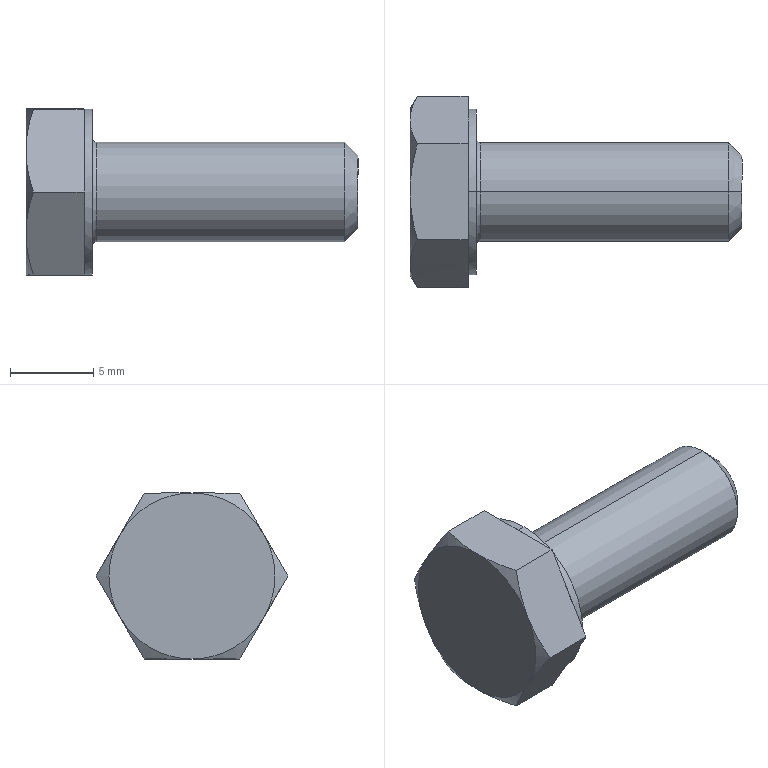Part | SolidWorks | features BaseBody 1 | 1 solid | 29 faces | box 20 x 11.547 x 10 mm | volume 788.422 mm3 | plane 15 | cone 8 | cylinder 4 | torus 2 | commonest cylinder face diameters 6 x2 10 x2
STEP:
#1=CARTESIAN_POINT('',(4.25,0.,3.));
#2=VERTEX_POINT('',#1);
#3=CARTESIAN_POINT('',(4.,0.,3.25));
#4=VERTEX_POINT('',#3);
#5=CARTESIAN_POINT('',(4.25,0.,3.25));
#6=DIRECTION('',(0.,1.,0.));
#7=DIRECTION('',(-1.,0.,0.));
#8=AXIS2_PLACEMENT_3D('',#5,#6,#7);
#9=CIRCLE('',#8,0.25);
#10=EDGE_CURVE('',#2,#4,#9,.T.);
#11=ORIENTED_EDGE('',*,*,#10,.F.);
#12=CARTESIAN_POINT('',(4.25,0.,-3.));
#13=VERTEX_POINT('',#12);
#14=CARTESIAN_POINT('',(4.25,0.,0.));
#15=DIRECTION('',(1.,0.,0.));
#16=DIRECTION('',(0.,0.,-1.));
#17=AXIS2_PLACEMENT_3D('',#14,#15,#16);
#18=CIRCLE('',#17,3.);
#19=EDGE_CURVE('',#13,#2,#18,.T.);
#20=ORIENTED_EDGE('',*,*,#19,.F.);
#21=CARTESIAN_POINT('',(4.,0.,-3.25));
#22=VERTEX_POINT('',#21);
#23=CARTESIAN_POINT('',(4.25,0.,-3.25));
#24=DIRECTION('',(0.,-1.,0.));
#25=DIRECTION('',(1.,0.,0.));
#26=AXIS2_PLACEMENT_3D('',#23,#24,#25);
#27=CIRCLE('',#26,0.25);
#28=EDGE_CURVE('',#13,#22,#27,.T.);
#29=ORIENTED_EDGE('',*,*,#28,.T.);
#30=CARTESIAN_POINT('',(4.,0.,0.));
#31=DIRECTION('',(-1.,0.,0.));
#32=DIRECTION('',(0.,0.,-1.));
#33=AXIS2_PLACEMENT_3D('',#30,#31,#32);
#34=CIRCLE('',#33,3.25);
#35=EDGE_CURVE('',#4,#22,#34,.T.);
#36=ORIENTED_EDGE('',*,*,#35,.F.);
#37=EDGE_LOOP('',(#11,#20,#29,#36));
#38=FACE_OUTER_BOUND('',#37,.T.);
#39=CARTESIAN_POINT('',(4.25,0.,0.));
#40=DIRECTION('',(1.,0.,0.));
#41=DIRECTION('',(0.,0.,-1.));
#42=AXIS2_PLACEMENT_3D('',#39,#40,#41);
#43=TOROIDAL_SURFACE('',#42,3.25,0.25);
#44=ADVANCED_FACE('',(#38),#43,.F.);
#45=CARTESIAN_POINT('',(20.,0.,-2.2));
#46=VERTEX_POINT('',#45);
#47=CARTESIAN_POINT('',(19.2,0.,-3.));
#48=VERTEX_POINT('',#47);
#49=CARTESIAN_POINT('',(19.2,0.,-3.));
#50=DIRECTION('',(-0.7071,0.,-0.7071));
#51=VECTOR('',#50,1000.);
#52=LINE('',#49,#51);
#53=EDGE_CURVE('',#46,#48,#52,.T.);
#54=ORIENTED_EDGE('',*,*,#53,.F.);
#55=CARTESIAN_POINT('',(20.,0.,2.2));
#56=VERTEX_POINT('',#55);
#57=CARTESIAN_POINT('',(20.,0.,0.));
#58=DIRECTION('',(1.,0.,0.));
#59=DIRECTION('',(0.,0.,1.));
#60=AXIS2_PLACEMENT_3D('',#57,#58,#59);
#61=CIRCLE('',#60,2.2);
#62=EDGE_CURVE('',#56,#46,#61,.T.);
#63=ORIENTED_EDGE('',*,*,#62,.F.);
#64=CARTESIAN_POINT('',(19.2,0.,3.));
#65=VERTEX_POINT('',#64);
#66=CARTESIAN_POINT('',(19.2,0.,3.));
#67=DIRECTION('',(-0.7071,0.,0.7071));
#68=VECTOR('',#67,1000.);
#69=LINE('',#66,#68);
#70=EDGE_CURVE('',#56,#65,#69,.T.);
#71=ORIENTED_EDGE('',*,*,#70,.T.);
#72=CARTESIAN_POINT('',(19.2,0.,0.));
#73=DIRECTION('',(-1.,0.,0.));
#74=DIRECTION('',(0.,0.,1.));
#75=AXIS2_PLACEMENT_3D('',#72,#73,#74);
#76=CIRCLE('',#75,3.);
#77=EDGE_CURVE('',#48,#65,#76,.T.);
#78=ORIENTED_EDGE('',*,*,#77,.F.);
#79=EDGE_LOOP('',(#54,#63,#71,#78));
#80=FACE_OUTER_BOUND('',#79,.T.);
#81=CARTESIAN_POINT('',(19.2,0.,0.));
#82=DIRECTION('',(-1.,0.,0.));
#83=DIRECTION('',(0.,0.,1.));
#84=AXIS2_PLACEMENT_3D('',#81,#82,#83);
#85=CONICAL_SURFACE('',#84,3.,0.7854);
#86=ADVANCED_FACE('',(#80),#85,.T.);
#87=CARTESIAN_POINT('',(4.,0.,0.));
#88=DIRECTION('',(-1.,0.,0.));
#89=DIRECTION('',(0.,0.,-1.));
#90=AXIS2_PLACEMENT_3D('',#87,#88,#89);
#91=CIRCLE('',#90,3.25);
#92=EDGE_CURVE('',#22,#4,#91,.T.);
#93=ORIENTED_EDGE('',*,*,#92,.T.);
#94=ORIENTED_EDGE('',*,*,#35,.T.);
#95=EDGE_LOOP('',(#93,#94));
#96=FACE_BOUND('',#95,.T.);
#97=CARTESIAN_POINT('',(4.,0.,5.));
#98=VERTEX_POINT('',#97);
#99=CARTESIAN_POINT('',(4.,0.,-5.));
#100=VERTEX_POINT('',#99);
#101=CARTESIAN_POINT('',(4.,0.,0.));
#102=DIRECTION('',(1.,0.,0.));
#103=DIRECTION('',(0.,0.,-1.));
#104=AXIS2_PLACEMENT_3D('',#101,#102,#103);
#105=CIRCLE('',#104,5.);
#106=EDGE_CURVE('',#98,#100,#105,.T.);
#107=ORIENTED_EDGE('',*,*,#106,.T.);
#108=CARTESIAN_POINT('',(4.,0.,0.));
#109=DIRECTION('',(1.,0.,0.));
#110=DIRECTION('',(0.,0.,-1.));
#111=AXIS2_PLACEMENT_3D('',#108,#109,#110);
#112=CIRCLE('',#111,5.);
#113=EDGE_CURVE('',#100,#98,#112,.T.);
#114=ORIENTED_EDGE('',*,*,#113,.T.);
#115=EDGE_LOOP('',(#107,#114));
#116=FACE_OUTER_BOUND('',#115,.T.);
#117=CARTESIAN_POINT('',(4.,0.,-10.));
#118=DIRECTION('',(1.,0.,0.));
#119=DIRECTION('',(0.,0.,-1.));
#120=AXIS2_PLACEMENT_3D('',#117,#118,#119);
#121=PLANE('',#120);
#122=ADVANCED_FACE('',(#96,#116),#121,.T.);
#123=CARTESIAN_POINT('',(0.,0.,-3.));
#124=DIRECTION('',(-1.,0.,0.));
#125=VECTOR('',#124,1000.);
#126=LINE('',#123,#125);
#127=EDGE_CURVE('',#48,#13,#126,.T.);
#128=ORIENTED_EDGE('',*,*,#127,.F.);
#129=ORIENTED_EDGE('',*,*,#77,.T.);
#130=CARTESIAN_POINT('',(0.,0.,3.));
#131=DIRECTION('',(-1.,0.,0.));
#132=VECTOR('',#131,1000.);
#133=LINE('',#130,#132);
#134=EDGE_CURVE('',#65,#2,#133,.T.);
#135=ORIENTED_EDGE('',*,*,#134,.T.);
#136=CARTESIAN_POINT('',(4.25,0.,0.));
#137=DIRECTION('',(1.,0.,0.));
#138=DIRECTION('',(0.,0.,-1.));
#139=AXIS2_PLACEMENT_3D('',#136,#137,#138);
#140=CIRCLE('',#139,3.);
#141=EDGE_CURVE('',#2,#13,#140,.T.);
#142=ORIENTED_EDGE('',*,*,#141,.T.);
#143=EDGE_LOOP('',(#128,#129,#135,#142));
#144=FACE_OUTER_BOUND('',#143,.T.);
#145=CARTESIAN_POINT('',(0.,0.,0.));
#146=DIRECTION('',(-1.,0.,0.));
#147=DIRECTION('',(0.,0.,1.));
#148=AXIS2_PLACEMENT_3D('',#145,#146,#147);
#149=CYLINDRICAL_SURFACE('',#148,3.);
#150=ADVANCED_FACE('',(#144),#149,.T.);
#151=ORIENTED_EDGE('',*,*,#62,.T.);
#152=CARTESIAN_POINT('',(20.,0.,0.));
#153=DIRECTION('',(1.,0.,0.));
#154=DIRECTION('',(0.,0.,1.));
#155=AXIS2_PLACEMENT_3D('',#152,#153,#154);
#156=CIRCLE('',#155,2.2);
#157=EDGE_CURVE('',#46,#56,#156,.T.);
#158=ORIENTED_EDGE('',*,*,#157,.T.);
#159=EDGE_LOOP('',(#151,#158));
#160=FACE_OUTER_BOUND('',#159,.T.);
#161=CARTESIAN_POINT('',(20.,0.,0.));
#162=DIRECTION('',(-1.,0.,0.));
#163=DIRECTION('',(0.,1.,0.));
#164=AXIS2_PLACEMENT_3D('',#161,#162,#163);
#165=PLANE('',#164);
#166=ADVANCED_FACE('',(#160),#165,.F.);
#167=CARTESIAN_POINT('',(3.5,0.,-5.));
#168=VERTEX_POINT('',#167);
#169=CARTESIAN_POINT('',(0.,0.,-5.));
#170=DIRECTION('',(-1.,0.,0.));
#171=VECTOR('',#170,1000.);
#172=LINE('',#169,#171);
#173=EDGE_CURVE('',#100,#168,#172,.T.);
#174=ORIENTED_EDGE('',*,*,#173,.F.);
#175=ORIENTED_EDGE('',*,*,#106,.F.);
#176=CARTESIAN_POINT('',(3.5,0.,5.));
#177=VERTEX_POINT('',#176);
#178=CARTESIAN_POINT('',(0.,0.,5.));
#179=DIRECTION('',(-1.,0.,0.));
#180=VECTOR('',#179,1000.);
#181=LINE('',#178,#180);
#182=EDGE_CURVE('',#98,#177,#181,.T.);
#183=ORIENTED_EDGE('',*,*,#182,.T.);
#184=CARTESIAN_POINT('',(3.5,-4.33,2.5));
#185=VERTEX_POINT('',#184);
#186=CARTESIAN_POINT('',(3.5,0.,0.));
#187=DIRECTION('',(-1.,0.,0.));
#188=DIRECTION('',(0.,0.,1.));
#189=AXIS2_PLACEMENT_3D('',#186,#187,#188);
#190=CIRCLE('',#189,5.);
#191=EDGE_CURVE('',#185,#177,#190,.T.);
#192=ORIENTED_EDGE('',*,*,#191,.F.);
#193=CARTESIAN_POINT('',(3.5,-4.33,-2.5));
#194=VERTEX_POINT('',#193);
#195=CARTESIAN_POINT('',(3.5,0.,0.));
#196=DIRECTION('',(-1.,0.,0.));
#197=DIRECTION('',(0.,0.,1.));
#198=AXIS2_PLACEMENT_3D('',#195,#196,#197);
#199=CIRCLE('',#198,5.);
#200=EDGE_CURVE('',#194,#185,#199,.T.);
#201=ORIENTED_EDGE('',*,*,#200,.F.);
#202=CARTESIAN_POINT('',(3.5,0.,0.));
#203=DIRECTION('',(-1.,0.,0.));
#204=DIRECTION('',(0.,0.,1.));
#205=AXIS2_PLACEMENT_3D('',#202,#203,#204);
#206=CIRCLE('',#205,5.);
#207=EDGE_CURVE('',#168,#194,#206,.T.);
#208=ORIENTED_EDGE('',*,*,#207,.F.);
#209=EDGE_LOOP('',(#174,#175,#183,#192,#201,#208));
#210=FACE_OUTER_BOUND('',#209,.T.);
#211=CARTESIAN_POINT('',(0.,0.,0.));
#212=DIRECTION('',(-1.,0.,0.));
#213=DIRECTION('',(0.,0.,1.));
#214=AXIS2_PLACEMENT_3D('',#211,#212,#213);
#215=CYLINDRICAL_SURFACE('',#214,5.);
#216=ADVANCED_FACE('',(#210),#215,.T.);
#217=CARTESIAN_POINT('',(3.5,-2.887,-5.));
#218=VERTEX_POINT('',#217);
#219=CARTESIAN_POINT('',(3.5,-2.887,-5.));
#220=DIRECTION('',(0.,0.5,-0.866));
#221=VECTOR('',#220,1000.);
#222=LINE('',#219,#221);
#223=EDGE_CURVE('',#194,#218,#222,.T.);
#224=ORIENTED_EDGE('',*,*,#223,.T.);
#225=CARTESIAN_POINT('',(3.5,2.887,-5.));
#226=DIRECTION('',(0.,1.,0.));
#227=VECTOR('',#226,1000.);
#228=LINE('',#225,#227);
#229=EDGE_CURVE('',#218,#168,#228,.T.);
#230=ORIENTED_EDGE('',*,*,#229,.T.);
#231=ORIENTED_EDGE('',*,*,#207,.T.);
#232=EDGE_LOOP('',(#224,#230,#231));
#233=FACE_OUTER_BOUND('',#232,.T.);
#234=CARTESIAN_POINT('',(3.5,5.,0.));
#235=DIRECTION('',(1.,0.,0.));
#236=DIRECTION('',(0.,0.,-1.));
#237=AXIS2_PLACEMENT_3D('',#234,#235,#236);
#238=PLANE('',#237);
#239=ADVANCED_FACE('',(#233),#238,.T.);
#240=CARTESIAN_POINT('',(3.5,-5.774,0.));
#241=VERTEX_POINT('',#240);
#242=CARTESIAN_POINT('',(3.5,-5.774,0.));
#243=DIRECTION('',(0.,-0.5,-0.866));
#244=VECTOR('',#243,1000.);
#245=LINE('',#242,#244);
#246=EDGE_CURVE('',#185,#241,#245,.T.);
#247=ORIENTED_EDGE('',*,*,#246,.T.);
#248=CARTESIAN_POINT('',(3.5,-2.887,-5.));
#249=DIRECTION('',(0.,0.5,-0.866));
#250=VECTOR('',#249,1000.);
#251=LINE('',#248,#250);
#252=EDGE_CURVE('',#241,#194,#251,.T.);
#253=ORIENTED_EDGE('',*,*,#252,.T.);
#254=ORIENTED_EDGE('',*,*,#200,.T.);
#255=EDGE_LOOP('',(#247,#253,#254));
#256=FACE_OUTER_BOUND('',#255,.T.);
#257=CARTESIAN_POINT('',(3.5,5.,0.));
#258=DIRECTION('',(1.,0.,0.));
#259=DIRECTION('',(0.,0.,-1.));
#260=AXIS2_PLACEMENT_3D('',#257,#258,#259);
#261=PLANE('',#260);
#262=ADVANCED_FACE('',(#256),#261,.T.);
#263=CARTESIAN_POINT('',(3.5,-2.887,5.));
#264=VERTEX_POINT('',#263);
#265=CARTESIAN_POINT('',(3.5,2.887,5.));
#266=DIRECTION('',(0.,-1.,0.));
#267=VECTOR('',#266,1000.);
#268=LINE('',#265,#267);
#269=EDGE_CURVE('',#177,#264,#268,.T.);
#270=ORIENTED_EDGE('',*,*,#269,.T.);
#271=CARTESIAN_POINT('',(3.5,-5.774,0.));
#272=DIRECTION('',(0.,-0.5,-0.866));
#273=VECTOR('',#272,1000.);
#274=LINE('',#271,#273);
#275=EDGE_CURVE('',#264,#185,#274,.T.);
#276=ORIENTED_EDGE('',*,*,#275,.T.);
#277=ORIENTED_EDGE('',*,*,#191,.T.);
#278=EDGE_LOOP('',(#270,#276,#277));
#279=FACE_OUTER_BOUND('',#278,.T.);
#280=CARTESIAN_POINT('',(3.5,5.,0.));
#281=DIRECTION('',(1.,0.,0.));
#282=DIRECTION('',(0.,0.,-1.));
#283=AXIS2_PLACEMENT_3D('',#280,#281,#282);
#284=PLANE('',#283);
#285=ADVANCED_FACE('',(#279),#284,.T.);
#286=CARTESIAN_POINT('',(3.5,4.33,2.5));
#287=VERTEX_POINT('',#286);
#288=CARTESIAN_POINT('',(3.5,2.887,5.));
#289=VERTEX_POINT('',#288);
#290=CARTESIAN_POINT('',(3.5,5.774,0.));
#291=DIRECTION('',(0.,-0.5,0.866));
#292=VECTOR('',#291,1000.);
#293=LINE('',#290,#292);
#294=EDGE_CURVE('',#287,#289,#293,.T.);
#295=ORIENTED_EDGE('',*,*,#294,.T.);
#296=CARTESIAN_POINT('',(3.5,2.887,5.));
#297=DIRECTION('',(0.,-1.,0.));
#298=VECTOR('',#297,1000.);
#299=LINE('',#296,#298);
#300=EDGE_CURVE('',#289,#177,#299,.T.);
#301=ORIENTED_EDGE('',*,*,#300,.T.);
#302=CARTESIAN_POINT('',(3.5,0.,0.));
#303=DIRECTION('',(-1.,0.,0.));
#304=DIRECTION('',(0.,0.,1.));
#305=AXIS2_PLACEMENT_3D('',#302,#303,#304);
#306=CIRCLE('',#305,5.);
#307=EDGE_CURVE('',#177,#287,#306,.T.);
#308=ORIENTED_EDGE('',*,*,#307,.T.);
#309=EDGE_LOOP('',(#295,#301,#308));
#310=FACE_OUTER_BOUND('',#309,.T.);
#311=CARTESIAN_POINT('',(3.5,5.,0.));
#312=DIRECTION('',(1.,0.,0.));
#313=DIRECTION('',(0.,0.,-1.));
#314=AXIS2_PLACEMENT_3D('',#311,#312,#313);
#315=PLANE('',#314);
#316=ADVANCED_FACE('',(#310),#315,.T.);
#317=CARTESIAN_POINT('',(3.5,4.33,-2.5));
#318=VERTEX_POINT('',#317);
#319=CARTESIAN_POINT('',(3.5,5.774,0.));
#320=VERTEX_POINT('',#319);
#321=CARTESIAN_POINT('',(3.5,2.887,-5.));
#322=DIRECTION('',(0.,0.5,0.866));
#323=VECTOR('',#322,1000.);
#324=LINE('',#321,#323);
#325=EDGE_CURVE('',#318,#320,#324,.T.);
#326=ORIENTED_EDGE('',*,*,#325,.T.);
#327=CARTESIAN_POINT('',(3.5,5.774,0.));
#328=DIRECTION('',(0.,-0.5,0.866));
#329=VECTOR('',#328,1000.);
#330=LINE('',#327,#329);
#331=EDGE_CURVE('',#320,#287,#330,.T.);
#332=ORIENTED_EDGE('',*,*,#331,.T.);
#333=CARTESIAN_POINT('',(3.5,0.,0.));
#334=DIRECTION('',(-1.,0.,0.));
#335=DIRECTION('',(0.,0.,1.));
#336=AXIS2_PLACEMENT_3D('',#333,#334,#335);
#337=CIRCLE('',#336,5.);
#338=EDGE_CURVE('',#287,#318,#337,.T.);
#339=ORIENTED_EDGE('',*,*,#338,.T.);
#340=EDGE_LOOP('',(#326,#332,#339));
#341=FACE_OUTER_BOUND('',#340,.T.);
#342=CARTESIAN_POINT('',(3.5,5.,0.));
#343=DIRECTION('',(1.,0.,0.));
#344=DIRECTION('',(0.,0.,-1.));
#345=AXIS2_PLACEMENT_3D('',#342,#343,#344);
#346=PLANE('',#345);
#347=ADVANCED_FACE('',(#341),#346,.T.);
#348=CARTESIAN_POINT('',(3.5,2.887,-5.));
#349=VERTEX_POINT('',#348);
#350=CARTESIAN_POINT('',(3.5,2.887,-5.));
#351=DIRECTION('',(0.,0.5,0.866));
#352=VECTOR('',#351,1000.);
#353=LINE('',#350,#352);
#354=EDGE_CURVE('',#349,#318,#353,.T.);
#355=ORIENTED_EDGE('',*,*,#354,.T.);
#356=CARTESIAN_POINT('',(3.5,0.,0.));
#357=DIRECTION('',(-1.,0.,0.));
#358=DIRECTION('',(0.,0.,1.));
#359=AXIS2_PLACEMENT_3D('',#356,#357,#358);
#360=CIRCLE('',#359,5.);
#361=EDGE_CURVE('',#318,#168,#360,.T.);
#362=ORIENTED_EDGE('',*,*,#361,.T.);
#363=CARTESIAN_POINT('',(3.5,2.887,-5.));
#364=DIRECTION('',(0.,1.,0.));
#365=VECTOR('',#364,1000.);
#366=LINE('',#363,#365);
#367=EDGE_CURVE('',#168,#349,#366,.T.);
#368=ORIENTED_EDGE('',*,*,#367,.T.);
#369=EDGE_LOOP('',(#355,#362,#368));
#370=FACE_OUTER_BOUND('',#369,.T.);
#371=CARTESIAN_POINT('',(3.5,5.,0.));
#372=DIRECTION('',(1.,0.,0.));
#373=DIRECTION('',(0.,0.,-1.));
#374=AXIS2_PLACEMENT_3D('',#371,#372,#373);
#375=PLANE('',#374);
#376=ADVANCED_FACE('',(#370),#375,.T.);
#377=CARTESIAN_POINT('',(0.,0.,-5.));
#378=VERTEX_POINT('',#377);
#379=CARTESIAN_POINT('',(0.,4.33,-2.5));
#380=VERTEX_POINT('',#379);
#381=CARTESIAN_POINT('',(0.,0.,0.));
#382=DIRECTION('',(1.,0.,0.));
#383=DIRECTION('',(0.,0.,-1.));
#384=AXIS2_PLACEMENT_3D('',#381,#382,#383);
#385=CIRCLE('',#384,5.);
#386=EDGE_CURVE('',#378,#380,#385,.T.);
#387=ORIENTED_EDGE('',*,*,#386,.F.);
#388=CARTESIAN_POINT('',(0.,-4.33,-2.5));
#389=VERTEX_POINT('',#388);
#390=CARTESIAN_POINT('',(0.,0.,0.));
#391=DIRECTION('',(1.,0.,0.));
#392=DIRECTION('',(0.,0.,-1.));
#393=AXIS2_PLACEMENT_3D('',#390,#391,#392);
#394=CIRCLE('',#393,5.);
#395=EDGE_CURVE('',#389,#378,#394,.T.);
#396=ORIENTED_EDGE('',*,*,#395,.F.);
#397=CARTESIAN_POINT('',(0.,-4.33,2.5));
#398=VERTEX_POINT('',#397);
#399=CARTESIAN_POINT('',(0.,0.,0.));
#400=DIRECTION('',(1.,0.,0.));
#401=DIRECTION('',(0.,0.,-1.));
#402=AXIS2_PLACEMENT_3D('',#399,#400,#401);
#403=CIRCLE('',#402,5.);
#404=EDGE_CURVE('',#398,#389,#403,.T.);
#405=ORIENTED_EDGE('',*,*,#404,.F.);
#406=CARTESIAN_POINT('',(0.,0.,5.));
#407=VERTEX_POINT('',#406);
#408=CARTESIAN_POINT('',(0.,0.,0.));
#409=DIRECTION('',(1.,0.,0.));
#410=DIRECTION('',(0.,0.,-1.));
#411=AXIS2_PLACEMENT_3D('',#408,#409,#410);
#412=CIRCLE('',#411,5.);
#413=EDGE_CURVE('',#407,#398,#412,.T.);
#414=ORIENTED_EDGE('',*,*,#413,.F.);
#415=CARTESIAN_POINT('',(0.,4.33,2.5));
#416=VERTEX_POINT('',#415);
#417=CARTESIAN_POINT('',(0.,0.,0.));
#418=DIRECTION('',(-1.,0.,0.));
#419=DIRECTION('',(0.,0.,1.));
#420=AXIS2_PLACEMENT_3D('',#417,#418,#419);
#421=CIRCLE('',#420,5.);
#422=EDGE_CURVE('',#407,#416,#421,.T.);
#423=ORIENTED_EDGE('',*,*,#422,.T.);
#424=CARTESIAN_POINT('',(0.,0.,0.));
#425=DIRECTION('',(1.,0.,0.));
#426=DIRECTION('',(0.,0.,-1.));
#427=AXIS2_PLACEMENT_3D('',#424,#425,#426);
#428=CIRCLE('',#427,5.);
#429=EDGE_CURVE('',#380,#416,#428,.T.);
#430=ORIENTED_EDGE('',*,*,#429,.F.);
#431=EDGE_LOOP('',(#387,#396,#405,#414,#423,#430));
#432=FACE_OUTER_BOUND('',#431,.T.);
#433=CARTESIAN_POINT('',(0.,0.,-10.));
#434=DIRECTION('',(1.,0.,0.));
#435=DIRECTION('',(0.,0.,-1.));
#436=AXIS2_PLACEMENT_3D('',#433,#434,#435);
#437=PLANE('',#436);
#438=ADVANCED_FACE('',(#432),#437,.F.);
#439=CARTESIAN_POINT('',(0.4466,2.887,-5.));
#440=VERTEX_POINT('',#439);
#441=CARTESIAN_POINT('',(0.,4.33,-2.5));
#442=CARTESIAN_POINT('',(0.,4.269,-2.606));
#443=CARTESIAN_POINT('',(0.002582,4.208,-2.712));
#444=CARTESIAN_POINT('',(0.01033,4.116,-2.871));
#445=CARTESIAN_POINT('',(0.01355,4.086,-2.924));
#446=CARTESIAN_POINT('',(0.0213,4.024,-3.03));
#447=CARTESIAN_POINT('',(0.02592,3.993,-3.084));
#448=CARTESIAN_POINT('',(0.04109,3.903,-3.24));
#449=CARTESIAN_POINT('',(0.05362,3.842,-3.345));
#450=CARTESIAN_POINT('',(0.07601,3.752,-3.502));
#451=CARTESIAN_POINT('',(0.08811,3.707,-3.58));
#452=CARTESIAN_POINT('',(0.1016,3.661,-3.659));
#453=CARTESIAN_POINT('',(0.1108,3.631,-3.712));
#454=CARTESIAN_POINT('',(0.1158,3.615,-3.739));
#455=CARTESIAN_POINT('',(0.196,3.367,-4.168));
#456=CARTESIAN_POINT('',(0.3047,3.133,-4.574));
#457=CARTESIAN_POINT('',(0.4466,2.887,-5.));
#458=B_SPLINE_CURVE_WITH_KNOTS('',3,(#441,#442,#443,#444,#445,#446,#447,#448,#449,#450,#451,#452,#453,#454,#455,#456,#457),.UNSPECIFIED.,.F.,.F.,(4,2,2,2,2,1,2,2,4),(0.,0.125,0.1875,0.25,0.375,0.4375,0.4687,0.5,1.),.UNSPECIFIED.);
#459=EDGE_CURVE('',#380,#440,#458,.T.);
#460=ORIENTED_EDGE('',*,*,#459,.T.);
#461=CARTESIAN_POINT('',(0.4466,2.887,-5.));
#462=CARTESIAN_POINT('',(0.3759,2.642,-5.));
#463=CARTESIAN_POINT('',(0.3135,2.403,-5.));
#464=CARTESIAN_POINT('',(0.2322,2.048,-5.));
#465=CARTESIAN_POINT('',(0.2072,1.931,-5.));
#466=CARTESIAN_POINT('',(0.1727,1.756,-5.));
#467=CARTESIAN_POINT('',(0.1562,1.669,-5.));
#468=CARTESIAN_POINT('',(0.1409,1.582,-5.));
#469=CARTESIAN_POINT('',(0.131,1.523,-5.));
#470=CARTESIAN_POINT('',(0.1264,1.496,-5.));
#471=CARTESIAN_POINT('',(0.1015,1.343,-5.));
#472=CARTESIAN_POINT('',(0.08408,1.221,-5.));
#473=CARTESIAN_POINT('',(0.05398,0.9783,-5.));
#474=CARTESIAN_POINT('',(0.04151,0.8589,-5.));
#475=CARTESIAN_POINT('',(0.01038,0.4883,-5.));
#476=CARTESIAN_POINT('',(0.,0.2449,-5.));
#477=CARTESIAN_POINT('',(0.,0.,-5.));
#478=B_SPLINE_CURVE_WITH_KNOTS('',3,(#461,#462,#463,#464,#465,#466,#467,#468,#469,#470,#471,#472,#473,#474,#475,#476,#477),.UNSPECIFIED.,.F.,.F.,(4,2,2,1,2,2,2,2,4),(0.,0.25,0.375,0.4375,0.4687,0.5,0.625,0.75,1.),.UNSPECIFIED.);
#479=EDGE_CURVE('',#440,#378,#478,.T.);
#480=ORIENTED_EDGE('',*,*,#479,.T.);
#481=ORIENTED_EDGE('',*,*,#386,.T.);
#482=EDGE_LOOP('',(#460,#480,#481));
#483=FACE_OUTER_BOUND('',#482,.T.);
#484=CARTESIAN_POINT('',(0.,0.,0.));
#485=DIRECTION('',(1.,0.,0.));
#486=DIRECTION('',(0.,0.,-1.));
#487=AXIS2_PLACEMENT_3D('',#484,#485,#486);
#488=CONICAL_SURFACE('',#487,5.,1.047);
#489=ADVANCED_FACE('',(#483),#488,.T.);
#490=CARTESIAN_POINT('',(0.4466,5.774,0.));
#491=VERTEX_POINT('',#490);
#492=CARTESIAN_POINT('',(0.,4.33,2.5));
#493=CARTESIAN_POINT('',(0.,4.391,2.394));
#494=CARTESIAN_POINT('',(0.002582,4.452,2.288));
#495=CARTESIAN_POINT('',(0.01033,4.544,2.129));
#496=CARTESIAN_POINT('',(0.01355,4.575,2.076));
#497=CARTESIAN_POINT('',(0.0213,4.636,1.97));
#498=CARTESIAN_POINT('',(0.02592,4.667,1.916));
#499=CARTESIAN_POINT('',(0.04109,4.758,1.76));
#500=CARTESIAN_POINT('',(0.05362,4.818,1.655));
#501=CARTESIAN_POINT('',(0.07601,4.908,1.498));
#502=CARTESIAN_POINT('',(0.08811,4.954,1.42));
#503=CARTESIAN_POINT('',(0.1016,4.999,1.341));
#504=CARTESIAN_POINT('',(0.1108,5.03,1.288));
#505=CARTESIAN_POINT('',(0.1158,5.046,1.261));
#506=CARTESIAN_POINT('',(0.196,5.293,0.8318));
#507=CARTESIAN_POINT('',(0.3047,5.528,0.4257));
#508=CARTESIAN_POINT('',(0.4466,5.774,0.));
#509=B_SPLINE_CURVE_WITH_KNOTS('',3,(#492,#493,#494,#495,#496,#497,#498,#499,#500,#501,#502,#503,#504,#505,#506,#507,#508),.UNSPECIFIED.,.F.,.F.,(4,2,2,2,2,1,2,2,4),(0.,0.125,0.1875,0.25,0.375,0.4375,0.4687,0.5,1.),.UNSPECIFIED.);
#510=EDGE_CURVE('',#416,#491,#509,.T.);
#511=ORIENTED_EDGE('',*,*,#510,.T.);
#512=CARTESIAN_POINT('',(0.4466,5.774,0.));
#513=CARTESIAN_POINT('',(0.3756,5.651,-0.2128));
#514=CARTESIAN_POINT('',(0.313,5.53,-0.421));
#515=CARTESIAN_POINT('',(0.2315,5.353,-0.7293));
#516=CARTESIAN_POINT('',(0.2063,5.294,-0.8314));
#517=CARTESIAN_POINT('',(0.1718,5.206,-0.984));
#518=CARTESIAN_POINT('',(0.1553,5.162,-1.06));
#519=CARTESIAN_POINT('',(0.14,5.118,-1.136));
#520=CARTESIAN_POINT('',(0.13,5.089,-1.187));
#521=CARTESIAN_POINT('',(0.1255,5.075,-1.21));
#522=CARTESIAN_POINT('',(0.04015,4.811,-1.668));
#523=CARTESIAN_POINT('',(0.,4.574,-2.078));
#524=CARTESIAN_POINT('',(0.,4.33,-2.5));
#525=B_SPLINE_CURVE_WITH_KNOTS('',3,(#512,#513,#514,#515,#516,#517,#518,#519,#520,#521,#522,#523,#524),.UNSPECIFIED.,.F.,.F.,(4,2,2,1,2,2,4),(0.,0.25,0.375,0.4375,0.4687,0.5,1.),.UNSPECIFIED.);
#526=EDGE_CURVE('',#491,#380,#525,.T.);
#527=ORIENTED_EDGE('',*,*,#526,.T.);
#528=ORIENTED_EDGE('',*,*,#429,.T.);
#529=EDGE_LOOP('',(#511,#527,#528));
#530=FACE_OUTER_BOUND('',#529,.T.);
#531=CARTESIAN_POINT('',(0.,0.,0.));
#532=DIRECTION('',(1.,0.,0.));
#533=DIRECTION('',(0.,0.,-1.));
#534=AXIS2_PLACEMENT_3D('',#531,#532,#533);
#535=CONICAL_SURFACE('',#534,5.,1.047);
#536=ADVANCED_FACE('',(#530),#535,.T.);
#537=CARTESIAN_POINT('',(0.4466,2.887,5.));
#538=VERTEX_POINT('',#537);
#539=CARTESIAN_POINT('',(0.,0.,5.));
#540=CARTESIAN_POINT('',(0.,0.1224,5.));
#541=CARTESIAN_POINT('',(0.002594,0.2445,5.));
#542=CARTESIAN_POINT('',(0.01297,0.4892,5.));
#543=CARTESIAN_POINT('',(0.02092,0.6138,5.));
#544=CARTESIAN_POINT('',(0.04135,0.8569,5.));
#545=CARTESIAN_POINT('',(0.05398,0.9782,5.));
#546=CARTESIAN_POINT('',(0.07655,1.16,5.));
#547=CARTESIAN_POINT('',(0.08874,1.252,5.));
#548=CARTESIAN_POINT('',(0.1023,1.343,5.));
#549=CARTESIAN_POINT('',(0.1116,1.404,5.));
#550=CARTESIAN_POINT('',(0.1167,1.436,5.));
#551=CARTESIAN_POINT('',(0.1968,1.93,5.));
#552=CARTESIAN_POINT('',(0.3052,2.397,5.));
#553=CARTESIAN_POINT('',(0.4466,2.887,5.));
#554=B_SPLINE_CURVE_WITH_KNOTS('',3,(#539,#540,#541,#542,#543,#544,#545,#546,#547,#548,#549,#550,#551,#552,#553),.UNSPECIFIED.,.F.,.F.,(4,2,2,2,1,2,2,4),(0.,0.125,0.25,0.375,0.4375,0.4688,0.5,1.),.UNSPECIFIED.);
#555=EDGE_CURVE('',#407,#538,#554,.T.);
#556=ORIENTED_EDGE('',*,*,#555,.T.);
#557=CARTESIAN_POINT('',(0.4466,2.887,5.));
#558=CARTESIAN_POINT('',(0.3756,3.01,4.787));
#559=CARTESIAN_POINT('',(0.313,3.13,4.579));
#560=CARTESIAN_POINT('',(0.2315,3.308,4.271));
#561=CARTESIAN_POINT('',(0.2063,3.367,4.169));
#562=CARTESIAN_POINT('',(0.1718,3.455,4.016));
#563=CARTESIAN_POINT('',(0.1553,3.499,3.94));
#564=CARTESIAN_POINT('',(0.14,3.543,3.864));
#565=CARTESIAN_POINT('',(0.13,3.572,3.814));
#566=CARTESIAN_POINT('',(0.1255,3.586,3.79));
#567=CARTESIAN_POINT('',(0.04015,3.85,3.333));
#568=CARTESIAN_POINT('',(0.,4.086,2.922));
#569=CARTESIAN_POINT('',(0.,4.33,2.5));
#570=B_SPLINE_CURVE_WITH_KNOTS('',3,(#557,#558,#559,#560,#561,#562,#563,#564,#565,#566,#567,#568,#569),.UNSPECIFIED.,.F.,.F.,(4,2,2,1,2,2,4),(0.,0.25,0.375,0.4375,0.4687,0.5,1.),.UNSPECIFIED.);
#571=EDGE_CURVE('',#538,#416,#570,.T.);
#572=ORIENTED_EDGE('',*,*,#571,.T.);
#573=ORIENTED_EDGE('',*,*,#422,.F.);
#574=EDGE_LOOP('',(#556,#572,#573));
#575=FACE_OUTER_BOUND('',#574,.T.);
#576=CARTESIAN_POINT('',(0.,0.,0.));
#577=DIRECTION('',(1.,0.,0.));
#578=DIRECTION('',(0.,0.,-1.));
#579=AXIS2_PLACEMENT_3D('',#576,#577,#578);
#580=CONICAL_SURFACE('',#579,5.,1.047);
#581=ADVANCED_FACE('',(#575),#580,.T.);
#582=CARTESIAN_POINT('',(0.4466,-2.887,5.));
#583=VERTEX_POINT('',#582);
#584=CARTESIAN_POINT('',(0.4466,-2.887,5.));
#585=CARTESIAN_POINT('',(0.3754,-2.64,5.));
#586=CARTESIAN_POINT('',(0.3125,-2.399,5.));
#587=CARTESIAN_POINT('',(0.2308,-2.042,5.));
#588=CARTESIAN_POINT('',(0.2056,-1.924,5.));
#589=CARTESIAN_POINT('',(0.171,-1.748,5.));
#590=CARTESIAN_POINT('',(0.1545,-1.66,5.));
#591=CARTESIAN_POINT('',(0.1392,-1.572,5.));
#592=CARTESIAN_POINT('',(0.1292,-1.513,5.));
#593=CARTESIAN_POINT('',(0.1246,-1.485,5.));
#594=CARTESIAN_POINT('',(0.1,-1.333,5.));
#595=CARTESIAN_POINT('',(0.08281,-1.212,5.));
#596=CARTESIAN_POINT('',(0.05313,-0.9707,5.));
#597=CARTESIAN_POINT('',(0.04083,-0.8523,5.));
#598=CARTESIAN_POINT('',(0.01021,-0.4851,5.));
#599=CARTESIAN_POINT('',(0.,-0.2435,5.));
#600=CARTESIAN_POINT('',(0.,0.,5.));
#601=B_SPLINE_CURVE_WITH_KNOTS('',3,(#584,#585,#586,#587,#588,#589,#590,#591,#592,#593,#594,#595,#596,#597,#598,#599,#600),.UNSPECIFIED.,.F.,.F.,(4,2,2,1,2,2,2,2,4),(0.,0.25,0.375,0.4375,0.4687,0.5,0.625,0.75,1.),.UNSPECIFIED.);
#602=EDGE_CURVE('',#583,#407,#601,.T.);
#603=ORIENTED_EDGE('',*,*,#602,.T.);
#604=ORIENTED_EDGE('',*,*,#413,.T.);
#605=CARTESIAN_POINT('',(0.,-4.33,2.5));
#606=CARTESIAN_POINT('',(0.,-4.269,2.606));
#607=CARTESIAN_POINT('',(0.002582,-4.208,2.712));
#608=CARTESIAN_POINT('',(0.01033,-4.116,2.871));
#609=CARTESIAN_POINT('',(0.01355,-4.086,2.924));
#610=CARTESIAN_POINT('',(0.0213,-4.024,3.03));
#611=CARTESIAN_POINT('',(0.02592,-3.993,3.084));
#612=CARTESIAN_POINT('',(0.04109,-3.903,3.24));
#613=CARTESIAN_POINT('',(0.05362,-3.842,3.345));
#614=CARTESIAN_POINT('',(0.07601,-3.752,3.502));
#615=CARTESIAN_POINT('',(0.08811,-3.707,3.58));
#616=CARTESIAN_POINT('',(0.1016,-3.661,3.659));
#617=CARTESIAN_POINT('',(0.1108,-3.631,3.712));
#618=CARTESIAN_POINT('',(0.1158,-3.615,3.739));
#619=CARTESIAN_POINT('',(0.196,-3.367,4.168));
#620=CARTESIAN_POINT('',(0.3047,-3.133,4.574));
#621=CARTESIAN_POINT('',(0.4466,-2.887,5.));
#622=B_SPLINE_CURVE_WITH_KNOTS('',3,(#605,#606,#607,#608,#609,#610,#611,#612,#613,#614,#615,#616,#617,#618,#619,#620,#621),.UNSPECIFIED.,.F.,.F.,(4,2,2,2,2,1,2,2,4),(0.,0.125,0.1875,0.25,0.375,0.4375,0.4687,0.5,1.),.UNSPECIFIED.);
#623=EDGE_CURVE('',#398,#583,#622,.T.);
#624=ORIENTED_EDGE('',*,*,#623,.T.);
#625=EDGE_LOOP('',(#603,#604,#624));
#626=FACE_OUTER_BOUND('',#625,.T.);
#627=CARTESIAN_POINT('',(0.,0.,0.));
#628=DIRECTION('',(1.,0.,0.));
#629=DIRECTION('',(0.,0.,-1.));
#630=AXIS2_PLACEMENT_3D('',#627,#628,#629);
#631=CONICAL_SURFACE('',#630,5.,1.047);
#632=ADVANCED_FACE('',(#626),#631,.T.);
#633=CARTESIAN_POINT('',(0.4466,-5.774,0.));
#634=VERTEX_POINT('',#633);
#635=CARTESIAN_POINT('',(0.4466,-5.774,0.));
#636=CARTESIAN_POINT('',(0.3756,-5.651,0.2128));
#637=CARTESIAN_POINT('',(0.313,-5.53,0.421));
#638=CARTESIAN_POINT('',(0.2315,-5.353,0.7293));
#639=CARTESIAN_POINT('',(0.2063,-5.294,0.8314));
#640=CARTESIAN_POINT('',(0.1718,-5.206,0.984));
#641=CARTESIAN_POINT('',(0.1553,-5.162,1.06));
#642=CARTESIAN_POINT('',(0.14,-5.118,1.136));
#643=CARTESIAN_POINT('',(0.13,-5.089,1.187));
#644=CARTESIAN_POINT('',(0.1255,-5.075,1.21));
#645=CARTESIAN_POINT('',(0.04015,-4.811,1.668));
#646=CARTESIAN_POINT('',(0.,-4.574,2.078));
#647=CARTESIAN_POINT('',(0.,-4.33,2.5));
#648=B_SPLINE_CURVE_WITH_KNOTS('',3,(#635,#636,#637,#638,#639,#640,#641,#642,#643,#644,#645,#646,#647),.UNSPECIFIED.,.F.,.F.,(4,2,2,1,2,2,4),(0.,0.25,0.375,0.4375,0.4687,0.5,1.),.UNSPECIFIED.);
#649=EDGE_CURVE('',#634,#398,#648,.T.);
#650=ORIENTED_EDGE('',*,*,#649,.T.);
#651=ORIENTED_EDGE('',*,*,#404,.T.);
#652=CARTESIAN_POINT('',(0.,-4.33,-2.5));
#653=CARTESIAN_POINT('',(0.,-4.391,-2.394));
#654=CARTESIAN_POINT('',(0.002582,-4.452,-2.288));
#655=CARTESIAN_POINT('',(0.01033,-4.544,-2.129));
#656=CARTESIAN_POINT('',(0.01355,-4.575,-2.076));
#657=CARTESIAN_POINT('',(0.0213,-4.636,-1.97));
#658=CARTESIAN_POINT('',(0.02592,-4.667,-1.916));
#659=CARTESIAN_POINT('',(0.04109,-4.758,-1.76));
#660=CARTESIAN_POINT('',(0.05362,-4.818,-1.655));
#661=CARTESIAN_POINT('',(0.07601,-4.908,-1.498));
#662=CARTESIAN_POINT('',(0.08811,-4.954,-1.42));
#663=CARTESIAN_POINT('',(0.1016,-4.999,-1.341));
#664=CARTESIAN_POINT('',(0.1108,-5.03,-1.288));
#665=CARTESIAN_POINT('',(0.1158,-5.046,-1.261));
#666=CARTESIAN_POINT('',(0.196,-5.293,-0.8318));
#667=CARTESIAN_POINT('',(0.3047,-5.528,-0.4257));
#668=CARTESIAN_POINT('',(0.4466,-5.774,0.));
#669=B_SPLINE_CURVE_WITH_KNOTS('',3,(#652,#653,#654,#655,#656,#657,#658,#659,#660,#661,#662,#663,#664,#665,#666,#667,#668),.UNSPECIFIED.,.F.,.F.,(4,2,2,2,2,1,2,2,4),(0.,0.125,0.1875,0.25,0.375,0.4375,0.4688,0.5,1.),.UNSPECIFIED.);
#670=EDGE_CURVE('',#389,#634,#669,.T.);
#671=ORIENTED_EDGE('',*,*,#670,.T.);
#672=EDGE_LOOP('',(#650,#651,#671));
#673=FACE_OUTER_BOUND('',#672,.T.);
#674=CARTESIAN_POINT('',(0.,0.,0.));
#675=DIRECTION('',(1.,0.,0.));
#676=DIRECTION('',(0.,0.,-1.));
#677=AXIS2_PLACEMENT_3D('',#674,#675,#676);
#678=CONICAL_SURFACE('',#677,5.,1.047);
#679=ADVANCED_FACE('',(#673),#678,.T.);
#680=CARTESIAN_POINT('',(0.4466,-2.887,-5.));
#681=VERTEX_POINT('',#680);
#682=CARTESIAN_POINT('',(0.4466,-2.887,-5.));
#683=CARTESIAN_POINT('',(0.3756,-3.01,-4.787));
#684=CARTESIAN_POINT('',(0.313,-3.13,-4.579));
#685=CARTESIAN_POINT('',(0.2315,-3.308,-4.271));
#686=CARTESIAN_POINT('',(0.2063,-3.367,-4.169));
#687=CARTESIAN_POINT('',(0.1718,-3.455,-4.016));
#688=CARTESIAN_POINT('',(0.1553,-3.499,-3.94));
#689=CARTESIAN_POINT('',(0.14,-3.543,-3.864));
#690=CARTESIAN_POINT('',(0.13,-3.572,-3.814));
#691=CARTESIAN_POINT('',(0.1255,-3.586,-3.79));
#692=CARTESIAN_POINT('',(0.04015,-3.85,-3.333));
#693=CARTESIAN_POINT('',(0.,-4.086,-2.922));
#694=CARTESIAN_POINT('',(0.,-4.33,-2.5));
#695=B_SPLINE_CURVE_WITH_KNOTS('',3,(#682,#683,#684,#685,#686,#687,#688,#689,#690,#691,#692,#693,#694),.UNSPECIFIED.,.F.,.F.,(4,2,2,1,2,2,4),(0.,0.25,0.375,0.4375,0.4688,0.5,1.),.UNSPECIFIED.);
#696=EDGE_CURVE('',#681,#389,#695,.T.);
#697=ORIENTED_EDGE('',*,*,#696,.T.);
#698=ORIENTED_EDGE('',*,*,#395,.T.);
#699=CARTESIAN_POINT('',(0.,0.,-5.));
#700=CARTESIAN_POINT('',(0.,-0.1217,-5.));
#701=CARTESIAN_POINT('',(0.002552,-0.243,-5.));
#702=CARTESIAN_POINT('',(0.01276,-0.4858,-5.));
#703=CARTESIAN_POINT('',(0.02057,-0.6093,-5.));
#704=CARTESIAN_POINT('',(0.04067,-0.8504,-5.));
#705=CARTESIAN_POINT('',(0.05312,-0.9707,-5.));
#706=CARTESIAN_POINT('',(0.07538,-1.152,-5.));
#707=CARTESIAN_POINT('',(0.08741,-1.242,-5.));
#708=CARTESIAN_POINT('',(0.1008,-1.333,-5.));
#709=CARTESIAN_POINT('',(0.11,-1.394,-5.));
#710=CARTESIAN_POINT('',(0.115,-1.425,-5.));
#711=CARTESIAN_POINT('',(0.1952,-1.923,-5.));
#712=CARTESIAN_POINT('',(0.3041,-2.393,-5.));
#713=CARTESIAN_POINT('',(0.4466,-2.887,-5.));
#714=B_SPLINE_CURVE_WITH_KNOTS('',3,(#699,#700,#701,#702,#703,#704,#705,#706,#707,#708,#709,#710,#711,#712,#713),.UNSPECIFIED.,.F.,.F.,(4,2,2,2,1,2,2,4),(0.,0.125,0.25,0.375,0.4375,0.4688,0.5,1.),.UNSPECIFIED.);
#715=EDGE_CURVE('',#378,#681,#714,.T.);
#716=ORIENTED_EDGE('',*,*,#715,.T.);
#717=EDGE_LOOP('',(#697,#698,#716));
#718=FACE_OUTER_BOUND('',#717,.T.);
#719=CARTESIAN_POINT('',(0.,0.,0.));
#720=DIRECTION('',(1.,0.,0.));
#721=DIRECTION('',(0.,0.,-1.));
#722=AXIS2_PLACEMENT_3D('',#719,#720,#721);
#723=CONICAL_SURFACE('',#722,5.,1.047);
#724=ADVANCED_FACE('',(#718),#723,.T.);
#725=ORIENTED_EDGE('',*,*,#229,.F.);
#726=CARTESIAN_POINT('',(4.,-2.887,-5.));
#727=DIRECTION('',(-1.,0.,0.));
#728=VECTOR('',#727,1000.);
#729=LINE('',#726,#728);
#730=EDGE_CURVE('',#218,#681,#729,.T.);
#731=ORIENTED_EDGE('',*,*,#730,.T.);
#732=ORIENTED_EDGE('',*,*,#715,.F.);
#733=ORIENTED_EDGE('',*,*,#479,.F.);
#734=CARTESIAN_POINT('',(4.,2.887,-5.));
#735=DIRECTION('',(-1.,0.,0.));
#736=VECTOR('',#735,1000.);
#737=LINE('',#734,#736);
#738=EDGE_CURVE('',#349,#440,#737,.T.);
#739=ORIENTED_EDGE('',*,*,#738,.F.);
#740=ORIENTED_EDGE('',*,*,#367,.F.);
#741=EDGE_LOOP('',(#725,#731,#732,#733,#739,#740));
#742=FACE_OUTER_BOUND('',#741,.T.);
#743=CARTESIAN_POINT('',(4.,2.887,-5.));
#744=DIRECTION('',(0.,0.,1.));
#745=DIRECTION('',(1.,0.,0.));
#746=AXIS2_PLACEMENT_3D('',#743,#744,#745);
#747=PLANE('',#746);
#748=ADVANCED_FACE('',(#742),#747,.F.);
#749=ORIENTED_EDGE('',*,*,#252,.F.);
#750=CARTESIAN_POINT('',(4.,-5.774,0.));
#751=DIRECTION('',(-1.,0.,0.));
#752=VECTOR('',#751,1000.);
#753=LINE('',#750,#752);
#754=EDGE_CURVE('',#241,#634,#753,.T.);
#755=ORIENTED_EDGE('',*,*,#754,.T.);
#756=ORIENTED_EDGE('',*,*,#670,.F.);
#757=ORIENTED_EDGE('',*,*,#696,.F.);
#758=ORIENTED_EDGE('',*,*,#730,.F.);
#759=ORIENTED_EDGE('',*,*,#223,.F.);
#760=EDGE_LOOP('',(#749,#755,#756,#757,#758,#759));
#761=FACE_OUTER_BOUND('',#760,.T.);
#762=CARTESIAN_POINT('',(4.,-2.887,-5.));
#763=DIRECTION('',(0.,0.866,0.5));
#764=DIRECTION('',(1.,0.,0.));
#765=AXIS2_PLACEMENT_3D('',#762,#763,#764);
#766=PLANE('',#765);
#767=ADVANCED_FACE('',(#761),#766,.F.);
#768=ORIENTED_EDGE('',*,*,#275,.F.);
#769=CARTESIAN_POINT('',(4.,-2.887,5.));
#770=DIRECTION('',(-1.,0.,0.));
#771=VECTOR('',#770,1000.);
#772=LINE('',#769,#771);
#773=EDGE_CURVE('',#264,#583,#772,.T.);
#774=ORIENTED_EDGE('',*,*,#773,.T.);
#775=ORIENTED_EDGE('',*,*,#623,.F.);
#776=ORIENTED_EDGE('',*,*,#649,.F.);
#777=ORIENTED_EDGE('',*,*,#754,.F.);
#778=ORIENTED_EDGE('',*,*,#246,.F.);
#779=EDGE_LOOP('',(#768,#774,#775,#776,#777,#778));
#780=FACE_OUTER_BOUND('',#779,.T.);
#781=CARTESIAN_POINT('',(4.,-5.774,0.));
#782=DIRECTION('',(0.,0.866,-0.5));
#783=DIRECTION('',(-1.,0.,0.));
#784=AXIS2_PLACEMENT_3D('',#781,#782,#783);
#785=PLANE('',#784);
#786=ADVANCED_FACE('',(#780),#785,.F.);
#787=ORIENTED_EDGE('',*,*,#300,.F.);
#788=CARTESIAN_POINT('',(4.,2.887,5.));
#789=DIRECTION('',(-1.,0.,0.));
#790=VECTOR('',#789,1000.);
#791=LINE('',#788,#790);
#792=EDGE_CURVE('',#289,#538,#791,.T.);
#793=ORIENTED_EDGE('',*,*,#792,.T.);
#794=ORIENTED_EDGE('',*,*,#555,.F.);
#795=ORIENTED_EDGE('',*,*,#602,.F.);
#796=ORIENTED_EDGE('',*,*,#773,.F.);
#797=ORIENTED_EDGE('',*,*,#269,.F.);
#798=EDGE_LOOP('',(#787,#793,#794,#795,#796,#797));
#799=FACE_OUTER_BOUND('',#798,.T.);
#800=CARTESIAN_POINT('',(4.,2.887,5.));
#801=DIRECTION('',(0.,0.,-1.));
#802=DIRECTION('',(0.,-1.,0.));
#803=AXIS2_PLACEMENT_3D('',#800,#801,#802);
#804=PLANE('',#803);
#805=ADVANCED_FACE('',(#799),#804,.F.);
#806=ORIENTED_EDGE('',*,*,#331,.F.);
#807=CARTESIAN_POINT('',(4.,5.774,0.));
#808=DIRECTION('',(-1.,0.,0.));
#809=VECTOR('',#808,1000.);
#810=LINE('',#807,#809);
#811=EDGE_CURVE('',#320,#491,#810,.T.);
#812=ORIENTED_EDGE('',*,*,#811,.T.);
#813=ORIENTED_EDGE('',*,*,#510,.F.);
#814=ORIENTED_EDGE('',*,*,#571,.F.);
#815=ORIENTED_EDGE('',*,*,#792,.F.);
#816=ORIENTED_EDGE('',*,*,#294,.F.);
#817=EDGE_LOOP('',(#806,#812,#813,#814,#815,#816));
#818=FACE_OUTER_BOUND('',#817,.T.);
#819=CARTESIAN_POINT('',(4.,5.774,0.));
#820=DIRECTION('',(0.,-0.866,-0.5));
#821=DIRECTION('',(0.,0.5,-0.866));
#822=AXIS2_PLACEMENT_3D('',#819,#820,#821);
#823=PLANE('',#822);
#824=ADVANCED_FACE('',(#818),#823,.F.);
#825=ORIENTED_EDGE('',*,*,#354,.F.);
#826=ORIENTED_EDGE('',*,*,#738,.T.);
#827=ORIENTED_EDGE('',*,*,#459,.F.);
#828=ORIENTED_EDGE('',*,*,#526,.F.);
#829=ORIENTED_EDGE('',*,*,#811,.F.);
#830=ORIENTED_EDGE('',*,*,#325,.F.);
#831=EDGE_LOOP('',(#825,#826,#827,#828,#829,#830));
#832=FACE_OUTER_BOUND('',#831,.T.);
#833=CARTESIAN_POINT('',(4.,2.887,-5.));
#834=DIRECTION('',(0.,-0.866,0.5));
#835=DIRECTION('',(-1.,0.,0.));
#836=AXIS2_PLACEMENT_3D('',#833,#834,#835);
#837=PLANE('',#836);
#838=ADVANCED_FACE('',(#832),#837,.F.);
#839=ORIENTED_EDGE('',*,*,#113,.F.);
#840=ORIENTED_EDGE('',*,*,#173,.T.);
#841=ORIENTED_EDGE('',*,*,#361,.F.);
#842=ORIENTED_EDGE('',*,*,#338,.F.);
#843=ORIENTED_EDGE('',*,*,#307,.F.);
#844=ORIENTED_EDGE('',*,*,#182,.F.);
#845=EDGE_LOOP('',(#839,#840,#841,#842,#843,#844));
#846=FACE_OUTER_BOUND('',#845,.T.);
#847=CARTESIAN_POINT('',(0.,0.,0.));
#848=DIRECTION('',(-1.,0.,0.));
#849=DIRECTION('',(0.,0.,1.));
#850=AXIS2_PLACEMENT_3D('',#847,#848,#849);
#851=CYLINDRICAL_SURFACE('',#850,5.);
#852=ADVANCED_FACE('',(#846),#851,.T.);
#853=CARTESIAN_POINT('',(19.2,0.,0.));
#854=DIRECTION('',(-1.,0.,0.));
#855=DIRECTION('',(0.,0.,1.));
#856=AXIS2_PLACEMENT_3D('',#853,#854,#855);
#857=CIRCLE('',#856,3.);
#858=EDGE_CURVE('',#65,#48,#857,.T.);
#859=ORIENTED_EDGE('',*,*,#858,.T.);
#860=ORIENTED_EDGE('',*,*,#127,.T.);
#861=ORIENTED_EDGE('',*,*,#19,.T.);
#862=ORIENTED_EDGE('',*,*,#134,.F.);
#863=EDGE_LOOP('',(#859,#860,#861,#862));
#864=FACE_OUTER_BOUND('',#863,.T.);
#865=CARTESIAN_POINT('',(0.,0.,0.));
#866=DIRECTION('',(-1.,0.,0.));
#867=DIRECTION('',(0.,0.,1.));
#868=AXIS2_PLACEMENT_3D('',#865,#866,#867);
#869=CYLINDRICAL_SURFACE('',#868,3.);
#870=ADVANCED_FACE('',(#864),#869,.T.);
#871=ORIENTED_EDGE('',*,*,#157,.F.);
#872=ORIENTED_EDGE('',*,*,#53,.T.);
#873=ORIENTED_EDGE('',*,*,#858,.F.);
#874=ORIENTED_EDGE('',*,*,#70,.F.);
#875=EDGE_LOOP('',(#871,#872,#873,#874));
#876=FACE_OUTER_BOUND('',#875,.T.);
#877=CARTESIAN_POINT('',(19.2,0.,0.));
#878=DIRECTION('',(-1.,0.,0.));
#879=DIRECTION('',(0.,0.,1.));
#880=AXIS2_PLACEMENT_3D('',#877,#878,#879);
#881=CONICAL_SURFACE('',#880,3.,0.7854);
#882=ADVANCED_FACE('',(#876),#881,.T.);
#883=ORIENTED_EDGE('',*,*,#141,.F.);
#884=ORIENTED_EDGE('',*,*,#10,.T.);
#885=ORIENTED_EDGE('',*,*,#92,.F.);
#886=ORIENTED_EDGE('',*,*,#28,.F.);
#887=EDGE_LOOP('',(#883,#884,#885,#886));
#888=FACE_OUTER_BOUND('',#887,.T.);
#889=CARTESIAN_POINT('',(4.25,0.,0.));
#890=DIRECTION('',(1.,0.,0.));
#891=DIRECTION('',(0.,0.,-1.));
#892=AXIS2_PLACEMENT_3D('',#889,#890,#891);
#893=TOROIDAL_SURFACE('',#892,3.25,0.25);
#894=ADVANCED_FACE('',(#888),#893,.F.);
#895=CLOSED_SHELL('',(#44,#86,#122,#150,#166,#216,#239,#262,#285,#316,#347,#376,#438,#489,#536,#581,#632,#679,#724,#748,#767,#786,#805,#824,#838,#852,#870,#882,#894));
#896=MANIFOLD_SOLID_BREP('',#895);
#897=CARTESIAN_POINT('',(0.,0.,0.));
#898=DIRECTION('',(0.,0.,1.));
#899=DIRECTION('',(1.,0.,0.));
#900=AXIS2_PLACEMENT_3D('',#897,#898,#899);
#901=(LENGTH_UNIT()NAMED_UNIT(*)SI_UNIT(.MILLI.,.METRE.));
#902=UNCERTAINTY_MEASURE_WITH_UNIT(LENGTH_MEASURE(0.00001),#901,'','');
#903=(NAMED_UNIT(*)PLANE_ANGLE_UNIT()SI_UNIT($,.RADIAN.));
#904=(NAMED_UNIT(*)SI_UNIT($,.STERADIAN.)SOLID_ANGLE_UNIT());
#905=(GEOMETRIC_REPRESENTATION_CONTEXT(3)GLOBAL_UNCERTAINTY_ASSIGNED_CONTEXT((#902))GLOBAL_UNIT_ASSIGNED_CONTEXT((#901,#903,#904))REPRESENTATION_CONTEXT('',''));
#906=ADVANCED_BREP_SHAPE_REPRESENTATION('',(#896,#900),#905);